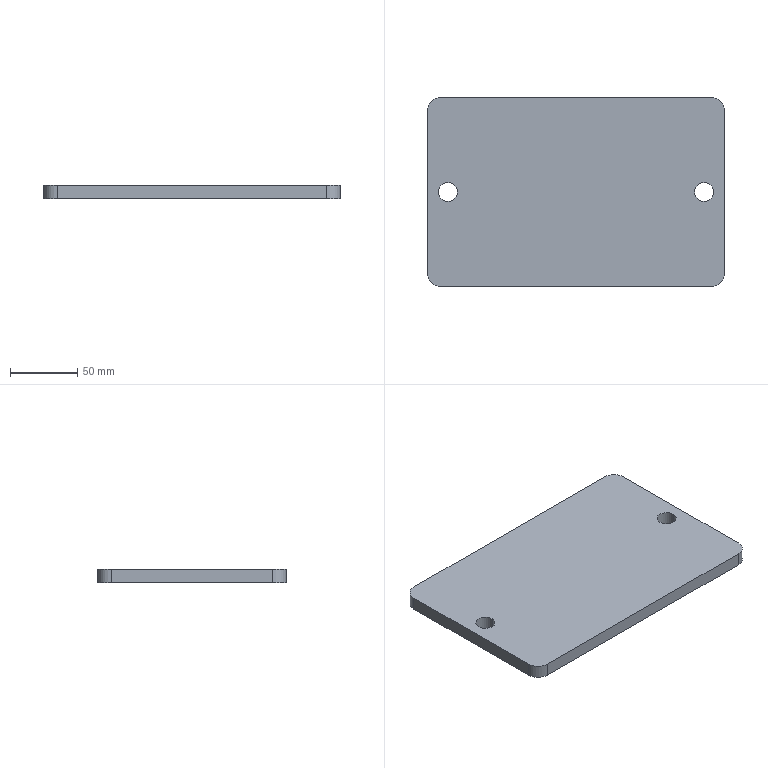Part | SolidWorks | features Extrusion 1, Fillet 1 | 1 solid | 14 faces | box 220 x 140 x 10 mm | volume 304063 mm3 | cylinder 8 | plane 6 | commonest cylinder face diameters 14 x4 20 x4
STEP:
#1=CARTESIAN_POINT('',(88.,0.,10.));
#2=VERTEX_POINT('',#1);
#3=CARTESIAN_POINT('',(102.,0.,10.));
#4=VERTEX_POINT('',#3);
#5=CARTESIAN_POINT('',(95.,0.,10.));
#6=DIRECTION('',(0.,0.,1.));
#7=DIRECTION('',(1.,0.,0.));
#8=AXIS2_PLACEMENT_3D('',#5,#6,#7);
#9=CIRCLE('',#8,7.);
#10=EDGE_CURVE('',#2,#4,#9,.T.);
#11=ORIENTED_EDGE('',*,*,#10,.T.);
#12=CARTESIAN_POINT('',(102.,0.,0.));
#13=VERTEX_POINT('',#12);
#14=CARTESIAN_POINT('',(102.,0.,10.));
#15=DIRECTION('',(0.,0.,-1.));
#16=VECTOR('',#15,1000.);
#17=LINE('',#14,#16);
#18=EDGE_CURVE('',#4,#13,#17,.T.);
#19=ORIENTED_EDGE('',*,*,#18,.T.);
#20=CARTESIAN_POINT('',(88.,0.,0.));
#21=VERTEX_POINT('',#20);
#22=CARTESIAN_POINT('',(95.,0.,0.));
#23=DIRECTION('',(0.,0.,1.));
#24=DIRECTION('',(1.,0.,0.));
#25=AXIS2_PLACEMENT_3D('',#22,#23,#24);
#26=CIRCLE('',#25,7.);
#27=EDGE_CURVE('',#21,#13,#26,.T.);
#28=ORIENTED_EDGE('',*,*,#27,.F.);
#29=CARTESIAN_POINT('',(88.,0.,10.));
#30=DIRECTION('',(0.,0.,-1.));
#31=VECTOR('',#30,1000.);
#32=LINE('',#29,#31);
#33=EDGE_CURVE('',#2,#21,#32,.T.);
#34=ORIENTED_EDGE('',*,*,#33,.F.);
#35=EDGE_LOOP('',(#11,#19,#28,#34));
#36=FACE_OUTER_BOUND('',#35,.T.);
#37=CARTESIAN_POINT('',(95.,0.,10.));
#38=DIRECTION('',(0.,0.,-1.));
#39=DIRECTION('',(-1.,0.,0.));
#40=AXIS2_PLACEMENT_3D('',#37,#38,#39);
#41=CYLINDRICAL_SURFACE('',#40,7.);
#42=ADVANCED_FACE('',(#36),#41,.F.);
#43=CARTESIAN_POINT('',(-102.,0.,10.));
#44=VERTEX_POINT('',#43);
#45=CARTESIAN_POINT('',(-88.,0.,10.));
#46=VERTEX_POINT('',#45);
#47=CARTESIAN_POINT('',(-95.,0.,10.));
#48=DIRECTION('',(0.,0.,1.));
#49=DIRECTION('',(1.,0.,0.));
#50=AXIS2_PLACEMENT_3D('',#47,#48,#49);
#51=CIRCLE('',#50,7.);
#52=EDGE_CURVE('',#44,#46,#51,.T.);
#53=ORIENTED_EDGE('',*,*,#52,.T.);
#54=CARTESIAN_POINT('',(-88.,0.,0.));
#55=VERTEX_POINT('',#54);
#56=CARTESIAN_POINT('',(-88.,0.,10.));
#57=DIRECTION('',(0.,0.,-1.));
#58=VECTOR('',#57,1000.);
#59=LINE('',#56,#58);
#60=EDGE_CURVE('',#46,#55,#59,.T.);
#61=ORIENTED_EDGE('',*,*,#60,.T.);
#62=CARTESIAN_POINT('',(-102.,0.,0.));
#63=VERTEX_POINT('',#62);
#64=CARTESIAN_POINT('',(-95.,0.,0.));
#65=DIRECTION('',(0.,0.,1.));
#66=DIRECTION('',(1.,0.,0.));
#67=AXIS2_PLACEMENT_3D('',#64,#65,#66);
#68=CIRCLE('',#67,7.);
#69=EDGE_CURVE('',#63,#55,#68,.T.);
#70=ORIENTED_EDGE('',*,*,#69,.F.);
#71=CARTESIAN_POINT('',(-102.,0.,10.));
#72=DIRECTION('',(0.,0.,-1.));
#73=VECTOR('',#72,1000.);
#74=LINE('',#71,#73);
#75=EDGE_CURVE('',#44,#63,#74,.T.);
#76=ORIENTED_EDGE('',*,*,#75,.F.);
#77=EDGE_LOOP('',(#53,#61,#70,#76));
#78=FACE_OUTER_BOUND('',#77,.T.);
#79=CARTESIAN_POINT('',(-95.,0.,10.));
#80=DIRECTION('',(0.,0.,-1.));
#81=DIRECTION('',(-1.,0.,0.));
#82=AXIS2_PLACEMENT_3D('',#79,#80,#81);
#83=CYLINDRICAL_SURFACE('',#82,7.);
#84=ADVANCED_FACE('',(#78),#83,.F.);
#85=CARTESIAN_POINT('',(-100.,-70.,10.));
#86=VERTEX_POINT('',#85);
#87=CARTESIAN_POINT('',(100.,-70.,10.));
#88=VERTEX_POINT('',#87);
#89=CARTESIAN_POINT('',(-110.,-70.,10.));
#90=DIRECTION('',(1.,0.,0.));
#91=VECTOR('',#90,1000.);
#92=LINE('',#89,#91);
#93=EDGE_CURVE('',#86,#88,#92,.T.);
#94=ORIENTED_EDGE('',*,*,#93,.T.);
#95=CARTESIAN_POINT('',(110.,-60.,10.));
#96=VERTEX_POINT('',#95);
#97=CARTESIAN_POINT('',(100.,-60.,10.));
#98=DIRECTION('',(0.,0.,1.));
#99=DIRECTION('',(-1.,0.,0.));
#100=AXIS2_PLACEMENT_3D('',#97,#98,#99);
#101=CIRCLE('',#100,10.);
#102=EDGE_CURVE('',#88,#96,#101,.T.);
#103=ORIENTED_EDGE('',*,*,#102,.T.);
#104=CARTESIAN_POINT('',(110.,60.,10.));
#105=VERTEX_POINT('',#104);
#106=CARTESIAN_POINT('',(110.,-70.,10.));
#107=DIRECTION('',(0.,1.,0.));
#108=VECTOR('',#107,1000.);
#109=LINE('',#106,#108);
#110=EDGE_CURVE('',#96,#105,#109,.T.);
#111=ORIENTED_EDGE('',*,*,#110,.T.);
#112=CARTESIAN_POINT('',(100.,70.,10.));
#113=VERTEX_POINT('',#112);
#114=CARTESIAN_POINT('',(100.,60.,10.));
#115=DIRECTION('',(0.,0.,1.));
#116=DIRECTION('',(-1.,0.,0.));
#117=AXIS2_PLACEMENT_3D('',#114,#115,#116);
#118=CIRCLE('',#117,10.);
#119=EDGE_CURVE('',#105,#113,#118,.T.);
#120=ORIENTED_EDGE('',*,*,#119,.T.);
#121=CARTESIAN_POINT('',(-100.,70.,10.));
#122=VERTEX_POINT('',#121);
#123=CARTESIAN_POINT('',(-110.,70.,10.));
#124=DIRECTION('',(-1.,0.,0.));
#125=VECTOR('',#124,1000.);
#126=LINE('',#123,#125);
#127=EDGE_CURVE('',#113,#122,#126,.T.);
#128=ORIENTED_EDGE('',*,*,#127,.T.);
#129=CARTESIAN_POINT('',(-110.,60.,10.));
#130=VERTEX_POINT('',#129);
#131=CARTESIAN_POINT('',(-100.,60.,10.));
#132=DIRECTION('',(0.,0.,1.));
#133=DIRECTION('',(-1.,0.,0.));
#134=AXIS2_PLACEMENT_3D('',#131,#132,#133);
#135=CIRCLE('',#134,10.);
#136=EDGE_CURVE('',#122,#130,#135,.T.);
#137=ORIENTED_EDGE('',*,*,#136,.T.);
#138=CARTESIAN_POINT('',(-110.,-60.,10.));
#139=VERTEX_POINT('',#138);
#140=CARTESIAN_POINT('',(-110.,-70.,10.));
#141=DIRECTION('',(0.,-1.,0.));
#142=VECTOR('',#141,1000.);
#143=LINE('',#140,#142);
#144=EDGE_CURVE('',#130,#139,#143,.T.);
#145=ORIENTED_EDGE('',*,*,#144,.T.);
#146=CARTESIAN_POINT('',(-100.,-60.,10.));
#147=DIRECTION('',(0.,0.,1.));
#148=DIRECTION('',(-1.,0.,0.));
#149=AXIS2_PLACEMENT_3D('',#146,#147,#148);
#150=CIRCLE('',#149,10.);
#151=EDGE_CURVE('',#139,#86,#150,.T.);
#152=ORIENTED_EDGE('',*,*,#151,.T.);
#153=EDGE_LOOP('',(#94,#103,#111,#120,#128,#137,#145,#152));
#154=FACE_OUTER_BOUND('',#153,.T.);
#155=ORIENTED_EDGE('',*,*,#52,.F.);
#156=CARTESIAN_POINT('',(-95.,0.,10.));
#157=DIRECTION('',(0.,0.,1.));
#158=DIRECTION('',(1.,0.,0.));
#159=AXIS2_PLACEMENT_3D('',#156,#157,#158);
#160=CIRCLE('',#159,7.);
#161=EDGE_CURVE('',#46,#44,#160,.T.);
#162=ORIENTED_EDGE('',*,*,#161,.F.);
#163=EDGE_LOOP('',(#155,#162));
#164=FACE_BOUND('',#163,.T.);
#165=ORIENTED_EDGE('',*,*,#10,.F.);
#166=CARTESIAN_POINT('',(95.,0.,10.));
#167=DIRECTION('',(0.,0.,1.));
#168=DIRECTION('',(1.,0.,0.));
#169=AXIS2_PLACEMENT_3D('',#166,#167,#168);
#170=CIRCLE('',#169,7.);
#171=EDGE_CURVE('',#4,#2,#170,.T.);
#172=ORIENTED_EDGE('',*,*,#171,.F.);
#173=EDGE_LOOP('',(#165,#172));
#174=FACE_BOUND('',#173,.T.);
#175=CARTESIAN_POINT('',(0.,0.,10.));
#176=DIRECTION('',(0.,0.,-1.));
#177=DIRECTION('',(-1.,0.,0.));
#178=AXIS2_PLACEMENT_3D('',#175,#176,#177);
#179=PLANE('',#178);
#180=ADVANCED_FACE('',(#154,#164,#174),#179,.F.);
#181=ORIENTED_EDGE('',*,*,#69,.T.);
#182=CARTESIAN_POINT('',(-95.,0.,0.));
#183=DIRECTION('',(0.,0.,1.));
#184=DIRECTION('',(1.,0.,0.));
#185=AXIS2_PLACEMENT_3D('',#182,#183,#184);
#186=CIRCLE('',#185,7.);
#187=EDGE_CURVE('',#55,#63,#186,.T.);
#188=ORIENTED_EDGE('',*,*,#187,.T.);
#189=EDGE_LOOP('',(#181,#188));
#190=FACE_BOUND('',#189,.T.);
#191=CARTESIAN_POINT('',(110.,-60.,0.));
#192=VERTEX_POINT('',#191);
#193=CARTESIAN_POINT('',(110.,60.,0.));
#194=VERTEX_POINT('',#193);
#195=CARTESIAN_POINT('',(110.,-70.,0.));
#196=DIRECTION('',(0.,1.,0.));
#197=VECTOR('',#196,1000.);
#198=LINE('',#195,#197);
#199=EDGE_CURVE('',#192,#194,#198,.T.);
#200=ORIENTED_EDGE('',*,*,#199,.F.);
#201=CARTESIAN_POINT('',(100.,-70.,0.));
#202=VERTEX_POINT('',#201);
#203=CARTESIAN_POINT('',(100.,-60.,0.));
#204=DIRECTION('',(0.,0.,-1.));
#205=DIRECTION('',(-1.,0.,0.));
#206=AXIS2_PLACEMENT_3D('',#203,#204,#205);
#207=CIRCLE('',#206,10.);
#208=EDGE_CURVE('',#192,#202,#207,.T.);
#209=ORIENTED_EDGE('',*,*,#208,.T.);
#210=CARTESIAN_POINT('',(-100.,-70.,0.));
#211=VERTEX_POINT('',#210);
#212=CARTESIAN_POINT('',(-110.,-70.,0.));
#213=DIRECTION('',(1.,0.,0.));
#214=VECTOR('',#213,1000.);
#215=LINE('',#212,#214);
#216=EDGE_CURVE('',#211,#202,#215,.T.);
#217=ORIENTED_EDGE('',*,*,#216,.F.);
#218=CARTESIAN_POINT('',(-110.,-60.,0.));
#219=VERTEX_POINT('',#218);
#220=CARTESIAN_POINT('',(-100.,-60.,0.));
#221=DIRECTION('',(0.,0.,-1.));
#222=DIRECTION('',(-1.,0.,0.));
#223=AXIS2_PLACEMENT_3D('',#220,#221,#222);
#224=CIRCLE('',#223,10.);
#225=EDGE_CURVE('',#211,#219,#224,.T.);
#226=ORIENTED_EDGE('',*,*,#225,.T.);
#227=CARTESIAN_POINT('',(-110.,60.,0.));
#228=VERTEX_POINT('',#227);
#229=CARTESIAN_POINT('',(-110.,-70.,0.));
#230=DIRECTION('',(0.,-1.,0.));
#231=VECTOR('',#230,1000.);
#232=LINE('',#229,#231);
#233=EDGE_CURVE('',#228,#219,#232,.T.);
#234=ORIENTED_EDGE('',*,*,#233,.F.);
#235=CARTESIAN_POINT('',(-100.,70.,0.));
#236=VERTEX_POINT('',#235);
#237=CARTESIAN_POINT('',(-100.,60.,0.));
#238=DIRECTION('',(0.,0.,-1.));
#239=DIRECTION('',(-1.,0.,0.));
#240=AXIS2_PLACEMENT_3D('',#237,#238,#239);
#241=CIRCLE('',#240,10.);
#242=EDGE_CURVE('',#228,#236,#241,.T.);
#243=ORIENTED_EDGE('',*,*,#242,.T.);
#244=CARTESIAN_POINT('',(100.,70.,0.));
#245=VERTEX_POINT('',#244);
#246=CARTESIAN_POINT('',(-110.,70.,0.));
#247=DIRECTION('',(-1.,0.,0.));
#248=VECTOR('',#247,1000.);
#249=LINE('',#246,#248);
#250=EDGE_CURVE('',#245,#236,#249,.T.);
#251=ORIENTED_EDGE('',*,*,#250,.F.);
#252=CARTESIAN_POINT('',(100.,60.,0.));
#253=DIRECTION('',(0.,0.,-1.));
#254=DIRECTION('',(-1.,0.,0.));
#255=AXIS2_PLACEMENT_3D('',#252,#253,#254);
#256=CIRCLE('',#255,10.);
#257=EDGE_CURVE('',#245,#194,#256,.T.);
#258=ORIENTED_EDGE('',*,*,#257,.T.);
#259=EDGE_LOOP('',(#200,#209,#217,#226,#234,#243,#251,#258));
#260=FACE_OUTER_BOUND('',#259,.T.);
#261=ORIENTED_EDGE('',*,*,#27,.T.);
#262=CARTESIAN_POINT('',(95.,0.,0.));
#263=DIRECTION('',(0.,0.,1.));
#264=DIRECTION('',(1.,0.,0.));
#265=AXIS2_PLACEMENT_3D('',#262,#263,#264);
#266=CIRCLE('',#265,7.);
#267=EDGE_CURVE('',#13,#21,#266,.T.);
#268=ORIENTED_EDGE('',*,*,#267,.T.);
#269=EDGE_LOOP('',(#261,#268));
#270=FACE_BOUND('',#269,.T.);
#271=CARTESIAN_POINT('',(0.,0.,0.));
#272=DIRECTION('',(0.,0.,-1.));
#273=DIRECTION('',(-1.,0.,0.));
#274=AXIS2_PLACEMENT_3D('',#271,#272,#273);
#275=PLANE('',#274);
#276=ADVANCED_FACE('',(#190,#260,#270),#275,.T.);
#277=ORIENTED_EDGE('',*,*,#233,.T.);
#278=CARTESIAN_POINT('',(-110.,-60.,10.));
#279=DIRECTION('',(0.,0.,1.));
#280=VECTOR('',#279,1000.);
#281=LINE('',#278,#280);
#282=EDGE_CURVE('',#219,#139,#281,.T.);
#283=ORIENTED_EDGE('',*,*,#282,.T.);
#284=ORIENTED_EDGE('',*,*,#144,.F.);
#285=CARTESIAN_POINT('',(-110.,60.,10.));
#286=DIRECTION('',(0.,0.,-1.));
#287=VECTOR('',#286,1000.);
#288=LINE('',#285,#287);
#289=EDGE_CURVE('',#130,#228,#288,.T.);
#290=ORIENTED_EDGE('',*,*,#289,.T.);
#291=EDGE_LOOP('',(#277,#283,#284,#290));
#292=FACE_OUTER_BOUND('',#291,.T.);
#293=CARTESIAN_POINT('',(-110.,-70.,10.));
#294=DIRECTION('',(1.,0.,0.));
#295=DIRECTION('',(0.,0.,-1.));
#296=AXIS2_PLACEMENT_3D('',#293,#294,#295);
#297=PLANE('',#296);
#298=ADVANCED_FACE('',(#292),#297,.F.);
#299=ORIENTED_EDGE('',*,*,#216,.T.);
#300=CARTESIAN_POINT('',(100.,-70.,10.));
#301=DIRECTION('',(0.,0.,1.));
#302=VECTOR('',#301,1000.);
#303=LINE('',#300,#302);
#304=EDGE_CURVE('',#202,#88,#303,.T.);
#305=ORIENTED_EDGE('',*,*,#304,.T.);
#306=ORIENTED_EDGE('',*,*,#93,.F.);
#307=CARTESIAN_POINT('',(-100.,-70.,10.));
#308=DIRECTION('',(0.,0.,-1.));
#309=VECTOR('',#308,1000.);
#310=LINE('',#307,#309);
#311=EDGE_CURVE('',#86,#211,#310,.T.);
#312=ORIENTED_EDGE('',*,*,#311,.T.);
#313=EDGE_LOOP('',(#299,#305,#306,#312));
#314=FACE_OUTER_BOUND('',#313,.T.);
#315=CARTESIAN_POINT('',(-110.,-70.,10.));
#316=DIRECTION('',(0.,1.,0.));
#317=DIRECTION('',(0.,0.,1.));
#318=AXIS2_PLACEMENT_3D('',#315,#316,#317);
#319=PLANE('',#318);
#320=ADVANCED_FACE('',(#314),#319,.F.);
#321=ORIENTED_EDGE('',*,*,#110,.F.);
#322=CARTESIAN_POINT('',(110.,-60.,10.));
#323=DIRECTION('',(0.,0.,-1.));
#324=VECTOR('',#323,1000.);
#325=LINE('',#322,#324);
#326=EDGE_CURVE('',#96,#192,#325,.T.);
#327=ORIENTED_EDGE('',*,*,#326,.T.);
#328=ORIENTED_EDGE('',*,*,#199,.T.);
#329=CARTESIAN_POINT('',(110.,60.,10.));
#330=DIRECTION('',(0.,0.,1.));
#331=VECTOR('',#330,1000.);
#332=LINE('',#329,#331);
#333=EDGE_CURVE('',#194,#105,#332,.T.);
#334=ORIENTED_EDGE('',*,*,#333,.T.);
#335=EDGE_LOOP('',(#321,#327,#328,#334));
#336=FACE_OUTER_BOUND('',#335,.T.);
#337=CARTESIAN_POINT('',(110.,-70.,10.));
#338=DIRECTION('',(-1.,0.,0.));
#339=DIRECTION('',(0.,0.,1.));
#340=AXIS2_PLACEMENT_3D('',#337,#338,#339);
#341=PLANE('',#340);
#342=ADVANCED_FACE('',(#336),#341,.F.);
#343=ORIENTED_EDGE('',*,*,#127,.F.);
#344=CARTESIAN_POINT('',(100.,70.,10.));
#345=DIRECTION('',(0.,0.,-1.));
#346=VECTOR('',#345,1000.);
#347=LINE('',#344,#346);
#348=EDGE_CURVE('',#113,#245,#347,.T.);
#349=ORIENTED_EDGE('',*,*,#348,.T.);
#350=ORIENTED_EDGE('',*,*,#250,.T.);
#351=CARTESIAN_POINT('',(-100.,70.,10.));
#352=DIRECTION('',(0.,0.,1.));
#353=VECTOR('',#352,1000.);
#354=LINE('',#351,#353);
#355=EDGE_CURVE('',#236,#122,#354,.T.);
#356=ORIENTED_EDGE('',*,*,#355,.T.);
#357=EDGE_LOOP('',(#343,#349,#350,#356));
#358=FACE_OUTER_BOUND('',#357,.T.);
#359=CARTESIAN_POINT('',(-110.,70.,10.));
#360=DIRECTION('',(0.,-1.,0.));
#361=DIRECTION('',(0.,0.,-1.));
#362=AXIS2_PLACEMENT_3D('',#359,#360,#361);
#363=PLANE('',#362);
#364=ADVANCED_FACE('',(#358),#363,.F.);
#365=ORIENTED_EDGE('',*,*,#60,.F.);
#366=ORIENTED_EDGE('',*,*,#161,.T.);
#367=ORIENTED_EDGE('',*,*,#75,.T.);
#368=ORIENTED_EDGE('',*,*,#187,.F.);
#369=EDGE_LOOP('',(#365,#366,#367,#368));
#370=FACE_OUTER_BOUND('',#369,.T.);
#371=CARTESIAN_POINT('',(-95.,0.,10.));
#372=DIRECTION('',(0.,0.,-1.));
#373=DIRECTION('',(-1.,0.,0.));
#374=AXIS2_PLACEMENT_3D('',#371,#372,#373);
#375=CYLINDRICAL_SURFACE('',#374,7.);
#376=ADVANCED_FACE('',(#370),#375,.F.);
#377=ORIENTED_EDGE('',*,*,#18,.F.);
#378=ORIENTED_EDGE('',*,*,#171,.T.);
#379=ORIENTED_EDGE('',*,*,#33,.T.);
#380=ORIENTED_EDGE('',*,*,#267,.F.);
#381=EDGE_LOOP('',(#377,#378,#379,#380));
#382=FACE_OUTER_BOUND('',#381,.T.);
#383=CARTESIAN_POINT('',(95.,0.,10.));
#384=DIRECTION('',(0.,0.,-1.));
#385=DIRECTION('',(-1.,0.,0.));
#386=AXIS2_PLACEMENT_3D('',#383,#384,#385);
#387=CYLINDRICAL_SURFACE('',#386,7.);
#388=ADVANCED_FACE('',(#382),#387,.F.);
#389=ORIENTED_EDGE('',*,*,#102,.F.);
#390=ORIENTED_EDGE('',*,*,#304,.F.);
#391=ORIENTED_EDGE('',*,*,#208,.F.);
#392=ORIENTED_EDGE('',*,*,#326,.F.);
#393=EDGE_LOOP('',(#389,#390,#391,#392));
#394=FACE_OUTER_BOUND('',#393,.T.);
#395=CARTESIAN_POINT('',(100.,-60.,10.));
#396=DIRECTION('',(0.,0.,-1.));
#397=DIRECTION('',(-1.,0.,0.));
#398=AXIS2_PLACEMENT_3D('',#395,#396,#397);
#399=CYLINDRICAL_SURFACE('',#398,10.);
#400=ADVANCED_FACE('',(#394),#399,.T.);
#401=ORIENTED_EDGE('',*,*,#151,.F.);
#402=ORIENTED_EDGE('',*,*,#282,.F.);
#403=ORIENTED_EDGE('',*,*,#225,.F.);
#404=ORIENTED_EDGE('',*,*,#311,.F.);
#405=EDGE_LOOP('',(#401,#402,#403,#404));
#406=FACE_OUTER_BOUND('',#405,.T.);
#407=CARTESIAN_POINT('',(-100.,-60.,10.));
#408=DIRECTION('',(0.,0.,-1.));
#409=DIRECTION('',(-1.,0.,0.));
#410=AXIS2_PLACEMENT_3D('',#407,#408,#409);
#411=CYLINDRICAL_SURFACE('',#410,10.);
#412=ADVANCED_FACE('',(#406),#411,.T.);
#413=ORIENTED_EDGE('',*,*,#119,.F.);
#414=ORIENTED_EDGE('',*,*,#333,.F.);
#415=ORIENTED_EDGE('',*,*,#257,.F.);
#416=ORIENTED_EDGE('',*,*,#348,.F.);
#417=EDGE_LOOP('',(#413,#414,#415,#416));
#418=FACE_OUTER_BOUND('',#417,.T.);
#419=CARTESIAN_POINT('',(100.,60.,10.));
#420=DIRECTION('',(0.,0.,-1.));
#421=DIRECTION('',(-1.,0.,0.));
#422=AXIS2_PLACEMENT_3D('',#419,#420,#421);
#423=CYLINDRICAL_SURFACE('',#422,10.);
#424=ADVANCED_FACE('',(#418),#423,.T.);
#425=ORIENTED_EDGE('',*,*,#136,.F.);
#426=ORIENTED_EDGE('',*,*,#355,.F.);
#427=ORIENTED_EDGE('',*,*,#242,.F.);
#428=ORIENTED_EDGE('',*,*,#289,.F.);
#429=EDGE_LOOP('',(#425,#426,#427,#428));
#430=FACE_OUTER_BOUND('',#429,.T.);
#431=CARTESIAN_POINT('',(-100.,60.,10.));
#432=DIRECTION('',(0.,0.,-1.));
#433=DIRECTION('',(-1.,0.,0.));
#434=AXIS2_PLACEMENT_3D('',#431,#432,#433);
#435=CYLINDRICAL_SURFACE('',#434,10.);
#436=ADVANCED_FACE('',(#430),#435,.T.);
#437=CLOSED_SHELL('',(#42,#84,#180,#276,#298,#320,#342,#364,#376,#388,#400,#412,#424,#436));
#438=MANIFOLD_SOLID_BREP('',#437);
#439=CARTESIAN_POINT('',(0.,0.,0.));
#440=DIRECTION('',(0.,0.,1.));
#441=DIRECTION('',(1.,0.,0.));
#442=AXIS2_PLACEMENT_3D('',#439,#440,#441);
#443=(LENGTH_UNIT()NAMED_UNIT(*)SI_UNIT(.MILLI.,.METRE.));
#444=UNCERTAINTY_MEASURE_WITH_UNIT(LENGTH_MEASURE(0.00001),#443,'','');
#445=(NAMED_UNIT(*)PLANE_ANGLE_UNIT()SI_UNIT($,.RADIAN.));
#446=(NAMED_UNIT(*)SI_UNIT($,.STERADIAN.)SOLID_ANGLE_UNIT());
#447=(GEOMETRIC_REPRESENTATION_CONTEXT(3)GLOBAL_UNCERTAINTY_ASSIGNED_CONTEXT((#444))GLOBAL_UNIT_ASSIGNED_CONTEXT((#443,#445,#446))REPRESENTATION_CONTEXT('',''));
#448=ADVANCED_BREP_SHAPE_REPRESENTATION('',(#438,#442),#447);